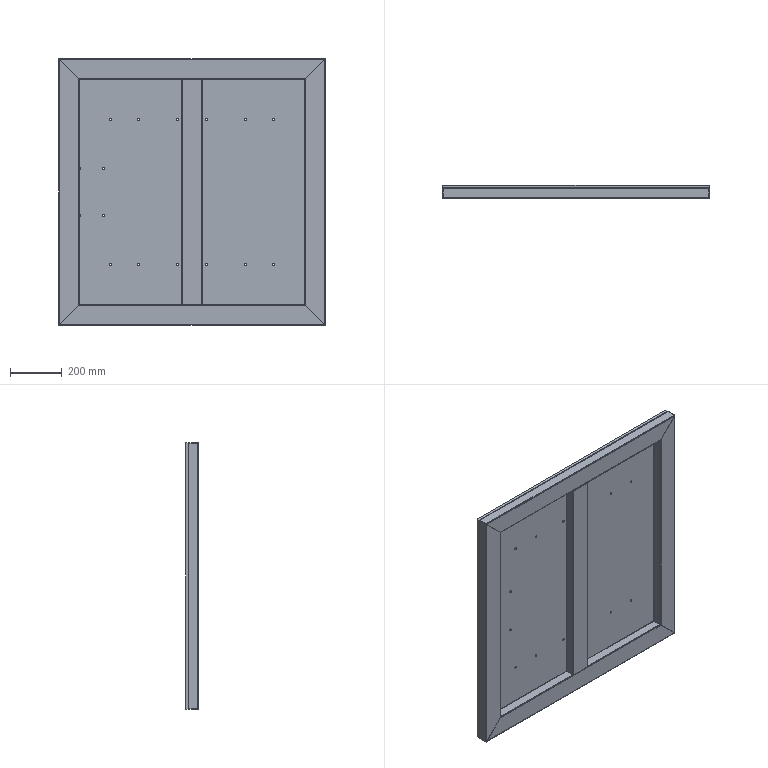Part | STEP file | 1-Base_default<welded> | 6 solids | 130 faces | box 1030 x 50 x 1030 mm | volume 12734708 mm3 | cylinder 72 | plane 56 | cone 2 | commonest cylinder face diameters 8.5 x32 2 x20 6 x20